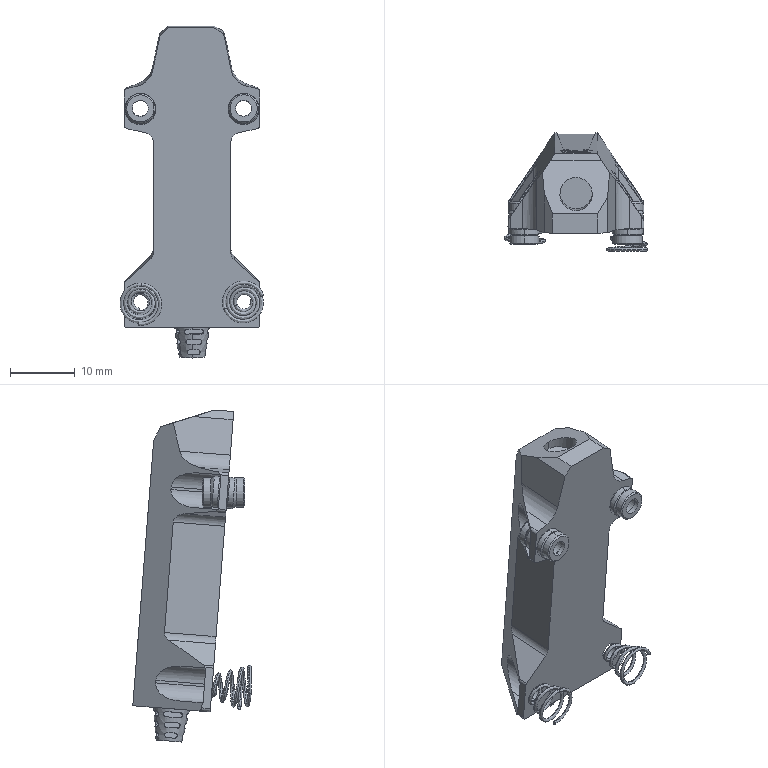Part | SolidWorks | features BaseBody 14 | 14 solids | 301 faces | box 22.271 x 18.317 x 51.362 mm | volume 5366 mm3 | plane 136 | cylinder 118 | cone 22 | spline 17 | sphere 8 | commonest cylinder face diameters 0.8 x36 2.8 x16 5 x10 1 x8 2.5 x8 4.6 x8